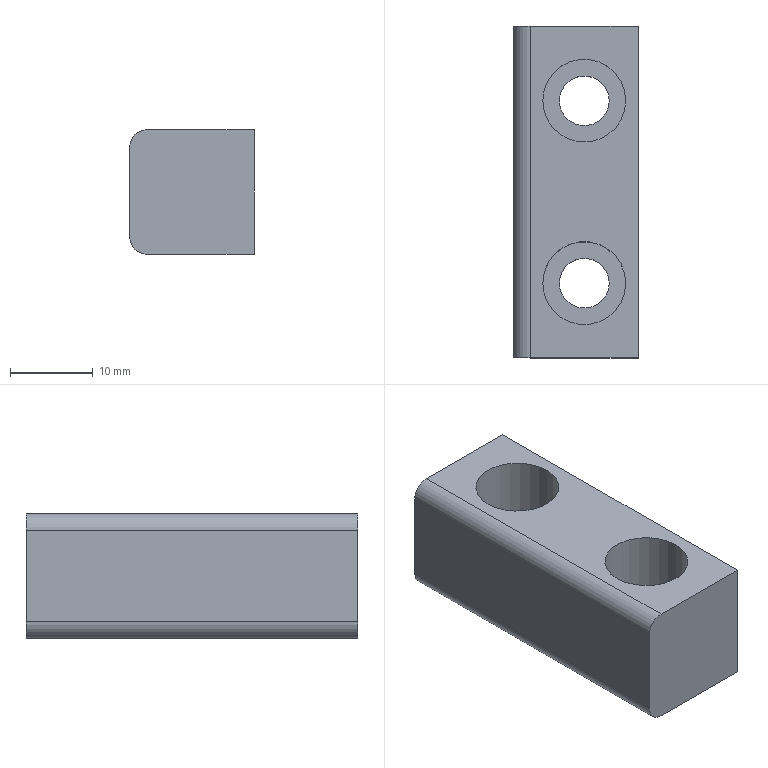Part | NX | features solid 2 | 1 solid | 14 faces | box 15 x 40 x 15 mm | volume 7279 mm3 | plane 8 | cylinder 6 | commonest cylinder face diameters 4 x2 6 x2 10 x2
STEP:
#1=CARTESIAN_POINT('',(496.902,-51.816,-17.));
#2=VERTEX_POINT('',#1);
#3=CARTESIAN_POINT('',(493.902,-51.816,-17.));
#4=DIRECTION('',(0.,0.,-1.));
#5=DIRECTION('',(1.,0.,0.));
#6=AXIS2_PLACEMENT_3D('',#3,#4,#5);
#7=CIRCLE('',#6,3.);
#8=EDGE_CURVE('',#2,#2,#7,.T.);
#9=ORIENTED_EDGE('',*,*,#8,.F.);
#10=EDGE_LOOP('',(#9));
#11=FACE_BOUND('',#10,.T.);
#12=CARTESIAN_POINT('',(487.402,-82.816,-17.));
#13=VERTEX_POINT('',#12);
#14=CARTESIAN_POINT('',(500.402,-82.816,-17.));
#15=VERTEX_POINT('',#14);
#16=CARTESIAN_POINT('',(490.402,-82.816,-17.));
#17=DIRECTION('',(1.,0.,0.));
#18=VECTOR('',#17,1000.);
#19=LINE('',#16,#18);
#20=EDGE_CURVE('',#13,#15,#19,.T.);
#21=ORIENTED_EDGE('',*,*,#20,.F.);
#22=CARTESIAN_POINT('',(487.402,-42.816,-17.));
#23=VERTEX_POINT('',#22);
#24=CARTESIAN_POINT('',(487.402,-62.816,-17.));
#25=DIRECTION('',(0.,-1.,0.));
#26=VECTOR('',#25,1000.);
#27=LINE('',#24,#26);
#28=EDGE_CURVE('',#13,#23,#27,.F.);
#29=ORIENTED_EDGE('',*,*,#28,.T.);
#30=CARTESIAN_POINT('',(500.402,-42.816,-17.));
#31=VERTEX_POINT('',#30);
#32=CARTESIAN_POINT('',(490.402,-42.816,-17.));
#33=DIRECTION('',(-1.,0.,0.));
#34=VECTOR('',#33,1000.);
#35=LINE('',#32,#34);
#36=EDGE_CURVE('',#31,#23,#35,.T.);
#37=ORIENTED_EDGE('',*,*,#36,.F.);
#38=CARTESIAN_POINT('',(500.402,-62.816,-17.));
#39=DIRECTION('',(0.,1.,0.));
#40=VECTOR('',#39,1000.);
#41=LINE('',#38,#40);
#42=EDGE_CURVE('',#15,#31,#41,.T.);
#43=ORIENTED_EDGE('',*,*,#42,.F.);
#44=EDGE_LOOP('',(#21,#29,#37,#43));
#45=FACE_BOUND('',#44,.T.);
#46=CARTESIAN_POINT('',(496.902,-73.816,-17.));
#47=VERTEX_POINT('',#46);
#48=CARTESIAN_POINT('',(493.902,-73.816,-17.));
#49=DIRECTION('',(0.,0.,1.));
#50=DIRECTION('',(1.,0.,0.));
#51=AXIS2_PLACEMENT_3D('',#48,#49,#50);
#52=CIRCLE('',#51,3.);
#53=EDGE_CURVE('',#47,#47,#52,.T.);
#54=ORIENTED_EDGE('',*,*,#53,.T.);
#55=EDGE_LOOP('',(#54));
#56=FACE_BOUND('',#55,.T.);
#57=CARTESIAN_POINT('',(490.402,-62.816,-17.));
#58=DIRECTION('',(0.,0.,-1.));
#59=DIRECTION('',(-1.,0.,0.));
#60=AXIS2_PLACEMENT_3D('',#57,#58,#59);
#61=PLANE('',#60);
#62=ADVANCED_FACE('',(#11,#45,#56),#61,.T.);
#63=CARTESIAN_POINT('',(498.902,-51.816,-2.));
#64=VERTEX_POINT('',#63);
#65=CARTESIAN_POINT('',(493.902,-51.816,-2.));
#66=DIRECTION('',(0.,0.,1.));
#67=DIRECTION('',(1.,0.,0.));
#68=AXIS2_PLACEMENT_3D('',#65,#66,#67);
#69=CIRCLE('',#68,5.);
#70=EDGE_CURVE('',#64,#64,#69,.T.);
#71=ORIENTED_EDGE('',*,*,#70,.F.);
#72=EDGE_LOOP('',(#71));
#73=FACE_BOUND('',#72,.T.);
#74=CARTESIAN_POINT('',(487.402,-42.816,-2.));
#75=VERTEX_POINT('',#74);
#76=CARTESIAN_POINT('',(500.402,-42.816,-2.));
#77=VERTEX_POINT('',#76);
#78=CARTESIAN_POINT('',(490.402,-42.816,-2.));
#79=DIRECTION('',(1.,0.,0.));
#80=VECTOR('',#79,1000.);
#81=LINE('',#78,#80);
#82=EDGE_CURVE('',#75,#77,#81,.T.);
#83=ORIENTED_EDGE('',*,*,#82,.F.);
#84=CARTESIAN_POINT('',(487.402,-82.816,-2.));
#85=VERTEX_POINT('',#84);
#86=CARTESIAN_POINT('',(487.402,-62.816,-2.));
#87=DIRECTION('',(0.,1.,0.));
#88=VECTOR('',#87,1000.);
#89=LINE('',#86,#88);
#90=EDGE_CURVE('',#75,#85,#89,.F.);
#91=ORIENTED_EDGE('',*,*,#90,.T.);
#92=CARTESIAN_POINT('',(500.402,-82.816,-2.));
#93=VERTEX_POINT('',#92);
#94=CARTESIAN_POINT('',(490.402,-82.816,-2.));
#95=DIRECTION('',(-1.,0.,0.));
#96=VECTOR('',#95,1000.);
#97=LINE('',#94,#96);
#98=EDGE_CURVE('',#93,#85,#97,.T.);
#99=ORIENTED_EDGE('',*,*,#98,.F.);
#100=CARTESIAN_POINT('',(500.402,-62.816,-2.));
#101=DIRECTION('',(0.,-1.,0.));
#102=VECTOR('',#101,1000.);
#103=LINE('',#100,#102);
#104=EDGE_CURVE('',#77,#93,#103,.T.);
#105=ORIENTED_EDGE('',*,*,#104,.F.);
#106=EDGE_LOOP('',(#83,#91,#99,#105));
#107=FACE_BOUND('',#106,.T.);
#108=CARTESIAN_POINT('',(498.902,-73.816,-2.));
#109=VERTEX_POINT('',#108);
#110=CARTESIAN_POINT('',(493.902,-73.816,-2.));
#111=DIRECTION('',(0.,0.,-1.));
#112=DIRECTION('',(1.,0.,0.));
#113=AXIS2_PLACEMENT_3D('',#110,#111,#112);
#114=CIRCLE('',#113,5.);
#115=EDGE_CURVE('',#109,#109,#114,.T.);
#116=ORIENTED_EDGE('',*,*,#115,.T.);
#117=EDGE_LOOP('',(#116));
#118=FACE_BOUND('',#117,.T.);
#119=CARTESIAN_POINT('',(490.402,-62.816,-2.));
#120=DIRECTION('',(0.,0.,1.));
#121=DIRECTION('',(1.,0.,0.));
#122=AXIS2_PLACEMENT_3D('',#119,#120,#121);
#123=PLANE('',#122);
#124=ADVANCED_FACE('',(#73,#107,#118),#123,.T.);
#125=CARTESIAN_POINT('',(485.402,-82.816,-15.));
#126=VERTEX_POINT('',#125);
#127=CARTESIAN_POINT('',(485.402,-82.816,-4.));
#128=VERTEX_POINT('',#127);
#129=CARTESIAN_POINT('',(485.402,-82.816,-12.));
#130=DIRECTION('',(0.,0.,1.));
#131=VECTOR('',#130,1000.);
#132=LINE('',#129,#131);
#133=EDGE_CURVE('',#126,#128,#132,.T.);
#134=ORIENTED_EDGE('',*,*,#133,.F.);
#135=CARTESIAN_POINT('',(487.402,-82.816,-15.));
#136=DIRECTION('',(0.,-1.,0.));
#137=DIRECTION('',(0.,0.,-1.));
#138=AXIS2_PLACEMENT_3D('',#135,#136,#137);
#139=CIRCLE('',#138,2.);
#140=EDGE_CURVE('',#126,#13,#139,.T.);
#141=ORIENTED_EDGE('',*,*,#140,.T.);
#142=ORIENTED_EDGE('',*,*,#20,.T.);
#143=CARTESIAN_POINT('',(500.402,-82.816,-12.));
#144=DIRECTION('',(0.,0.,1.));
#145=VECTOR('',#144,1000.);
#146=LINE('',#143,#145);
#147=EDGE_CURVE('',#15,#93,#146,.T.);
#148=ORIENTED_EDGE('',*,*,#147,.T.);
#149=ORIENTED_EDGE('',*,*,#98,.T.);
#150=CARTESIAN_POINT('',(487.402,-82.816,-4.));
#151=DIRECTION('',(0.,-1.,0.));
#152=DIRECTION('',(0.,0.,-1.));
#153=AXIS2_PLACEMENT_3D('',#150,#151,#152);
#154=CIRCLE('',#153,2.);
#155=EDGE_CURVE('',#85,#128,#154,.T.);
#156=ORIENTED_EDGE('',*,*,#155,.T.);
#157=EDGE_LOOP('',(#134,#141,#142,#148,#149,#156));
#158=FACE_BOUND('',#157,.T.);
#159=CARTESIAN_POINT('',(490.402,-82.816,-12.));
#160=DIRECTION('',(0.,-1.,0.));
#161=DIRECTION('',(0.,0.,-1.));
#162=AXIS2_PLACEMENT_3D('',#159,#160,#161);
#163=PLANE('',#162);
#164=ADVANCED_FACE('',(#158),#163,.T.);
#165=CARTESIAN_POINT('',(485.402,-42.816,-15.));
#166=VERTEX_POINT('',#165);
#167=CARTESIAN_POINT('',(485.402,-42.816,-4.));
#168=VERTEX_POINT('',#167);
#169=CARTESIAN_POINT('',(485.402,-42.816,-12.));
#170=DIRECTION('',(0.,0.,1.));
#171=VECTOR('',#170,1000.);
#172=LINE('',#169,#171);
#173=EDGE_CURVE('',#166,#168,#172,.T.);
#174=ORIENTED_EDGE('',*,*,#173,.F.);
#175=CARTESIAN_POINT('',(485.402,-62.816,-15.));
#176=DIRECTION('',(0.,-1.,0.));
#177=VECTOR('',#176,1000.);
#178=LINE('',#175,#177);
#179=EDGE_CURVE('',#166,#126,#178,.T.);
#180=ORIENTED_EDGE('',*,*,#179,.T.);
#181=ORIENTED_EDGE('',*,*,#133,.T.);
#182=CARTESIAN_POINT('',(485.402,-62.816,-4.));
#183=DIRECTION('',(0.,1.,0.));
#184=VECTOR('',#183,1000.);
#185=LINE('',#182,#184);
#186=EDGE_CURVE('',#128,#168,#185,.T.);
#187=ORIENTED_EDGE('',*,*,#186,.T.);
#188=EDGE_LOOP('',(#174,#180,#181,#187));
#189=FACE_BOUND('',#188,.T.);
#190=CARTESIAN_POINT('',(485.402,-62.816,-12.));
#191=DIRECTION('',(-1.,0.,0.));
#192=DIRECTION('',(0.,0.,1.));
#193=AXIS2_PLACEMENT_3D('',#190,#191,#192);
#194=PLANE('',#193);
#195=ADVANCED_FACE('',(#189),#194,.T.);
#196=ORIENTED_EDGE('',*,*,#36,.T.);
#197=CARTESIAN_POINT('',(487.402,-42.816,-15.));
#198=DIRECTION('',(0.,1.,0.));
#199=DIRECTION('',(0.,0.,1.));
#200=AXIS2_PLACEMENT_3D('',#197,#198,#199);
#201=CIRCLE('',#200,2.);
#202=EDGE_CURVE('',#23,#166,#201,.T.);
#203=ORIENTED_EDGE('',*,*,#202,.T.);
#204=ORIENTED_EDGE('',*,*,#173,.T.);
#205=CARTESIAN_POINT('',(487.402,-42.816,-4.));
#206=DIRECTION('',(0.,1.,0.));
#207=DIRECTION('',(0.,0.,1.));
#208=AXIS2_PLACEMENT_3D('',#205,#206,#207);
#209=CIRCLE('',#208,2.);
#210=EDGE_CURVE('',#168,#75,#209,.T.);
#211=ORIENTED_EDGE('',*,*,#210,.T.);
#212=ORIENTED_EDGE('',*,*,#82,.T.);
#213=CARTESIAN_POINT('',(500.402,-42.816,-12.));
#214=DIRECTION('',(0.,0.,1.));
#215=VECTOR('',#214,1000.);
#216=LINE('',#213,#215);
#217=EDGE_CURVE('',#31,#77,#216,.T.);
#218=ORIENTED_EDGE('',*,*,#217,.F.);
#219=EDGE_LOOP('',(#196,#203,#204,#211,#212,#218));
#220=FACE_BOUND('',#219,.T.);
#221=CARTESIAN_POINT('',(490.402,-42.816,-12.));
#222=DIRECTION('',(0.,1.,0.));
#223=DIRECTION('',(0.,0.,1.));
#224=AXIS2_PLACEMENT_3D('',#221,#222,#223);
#225=PLANE('',#224);
#226=ADVANCED_FACE('',(#220),#225,.T.);
#227=ORIENTED_EDGE('',*,*,#42,.T.);
#228=ORIENTED_EDGE('',*,*,#217,.T.);
#229=ORIENTED_EDGE('',*,*,#104,.T.);
#230=ORIENTED_EDGE('',*,*,#147,.F.);
#231=EDGE_LOOP('',(#227,#228,#229,#230));
#232=FACE_BOUND('',#231,.T.);
#233=CARTESIAN_POINT('',(500.402,-62.816,-12.));
#234=DIRECTION('',(1.,0.,0.));
#235=DIRECTION('',(0.,0.,-1.));
#236=AXIS2_PLACEMENT_3D('',#233,#234,#235);
#237=PLANE('',#236);
#238=ADVANCED_FACE('',(#232),#237,.T.);
#239=ORIENTED_EDGE('',*,*,#202,.F.);
#240=ORIENTED_EDGE('',*,*,#28,.F.);
#241=ORIENTED_EDGE('',*,*,#140,.F.);
#242=ORIENTED_EDGE('',*,*,#179,.F.);
#243=EDGE_LOOP('',(#239,#240,#241,#242));
#244=FACE_BOUND('',#243,.T.);
#245=CARTESIAN_POINT('',(487.402,-62.816,-15.));
#246=DIRECTION('',(0.,-1.,0.));
#247=DIRECTION('',(0.,0.,-1.));
#248=AXIS2_PLACEMENT_3D('',#245,#246,#247);
#249=CYLINDRICAL_SURFACE('',#248,2.);
#250=ADVANCED_FACE('',(#244),#249,.T.);
#251=ORIENTED_EDGE('',*,*,#155,.F.);
#252=ORIENTED_EDGE('',*,*,#90,.F.);
#253=ORIENTED_EDGE('',*,*,#210,.F.);
#254=ORIENTED_EDGE('',*,*,#186,.F.);
#255=EDGE_LOOP('',(#251,#252,#253,#254));
#256=FACE_BOUND('',#255,.T.);
#257=CARTESIAN_POINT('',(487.402,-62.816,-4.));
#258=DIRECTION('',(0.,1.,0.));
#259=DIRECTION('',(0.,0.,1.));
#260=AXIS2_PLACEMENT_3D('',#257,#258,#259);
#261=CYLINDRICAL_SURFACE('',#260,2.);
#262=ADVANCED_FACE('',(#256),#261,.T.);
#263=CARTESIAN_POINT('',(490.902,-73.816,-10.));
#264=VERTEX_POINT('',#263);
#265=CARTESIAN_POINT('',(493.902,-73.816,-10.));
#266=DIRECTION('',(0.,0.,-1.));
#267=DIRECTION('',(-1.,0.,0.));
#268=AXIS2_PLACEMENT_3D('',#265,#266,#267);
#269=CIRCLE('',#268,3.);
#270=EDGE_CURVE('',#264,#264,#269,.T.);
#271=ORIENTED_EDGE('',*,*,#270,.F.);
#272=EDGE_LOOP('',(#271));
#273=FACE_BOUND('',#272,.T.);
#274=ORIENTED_EDGE('',*,*,#53,.F.);
#275=EDGE_LOOP('',(#274));
#276=FACE_BOUND('',#275,.T.);
#277=CARTESIAN_POINT('',(493.902,-73.816,-2.));
#278=DIRECTION('',(0.,0.,-1.));
#279=DIRECTION('',(1.,0.,0.));
#280=AXIS2_PLACEMENT_3D('',#277,#278,#279);
#281=CYLINDRICAL_SURFACE('',#280,3.);
#282=ADVANCED_FACE('',(#273,#276),#281,.F.);
#283=ORIENTED_EDGE('',*,*,#270,.T.);
#284=EDGE_LOOP('',(#283));
#285=FACE_BOUND('',#284,.T.);
#286=CARTESIAN_POINT('',(498.902,-73.816,-10.));
#287=VERTEX_POINT('',#286);
#288=CARTESIAN_POINT('',(493.902,-73.816,-10.));
#289=DIRECTION('',(0.,0.,1.));
#290=DIRECTION('',(1.,0.,0.));
#291=AXIS2_PLACEMENT_3D('',#288,#289,#290);
#292=CIRCLE('',#291,5.);
#293=EDGE_CURVE('',#287,#287,#292,.F.);
#294=ORIENTED_EDGE('',*,*,#293,.F.);
#295=EDGE_LOOP('',(#294));
#296=FACE_BOUND('',#295,.T.);
#297=CARTESIAN_POINT('',(493.902,-73.816,-10.));
#298=DIRECTION('',(0.,0.,-1.));
#299=DIRECTION('',(-1.,0.,0.));
#300=AXIS2_PLACEMENT_3D('',#297,#298,#299);
#301=PLANE('',#300);
#302=ADVANCED_FACE('',(#285,#296),#301,.F.);
#303=ORIENTED_EDGE('',*,*,#293,.T.);
#304=EDGE_LOOP('',(#303));
#305=FACE_BOUND('',#304,.T.);
#306=ORIENTED_EDGE('',*,*,#115,.F.);
#307=EDGE_LOOP('',(#306));
#308=FACE_BOUND('',#307,.T.);
#309=CARTESIAN_POINT('',(493.902,-73.816,-2.));
#310=DIRECTION('',(0.,0.,-1.));
#311=DIRECTION('',(1.,0.,0.));
#312=AXIS2_PLACEMENT_3D('',#309,#310,#311);
#313=CYLINDRICAL_SURFACE('',#312,5.);
#314=ADVANCED_FACE('',(#305,#308),#313,.F.);
#315=CARTESIAN_POINT('',(490.902,-51.816,-10.));
#316=VERTEX_POINT('',#315);
#317=CARTESIAN_POINT('',(493.902,-51.816,-10.));
#318=DIRECTION('',(0.,0.,1.));
#319=DIRECTION('',(-1.,0.,0.));
#320=AXIS2_PLACEMENT_3D('',#317,#318,#319);
#321=CIRCLE('',#320,3.);
#322=EDGE_CURVE('',#316,#316,#321,.T.);
#323=ORIENTED_EDGE('',*,*,#322,.T.);
#324=EDGE_LOOP('',(#323));
#325=FACE_BOUND('',#324,.T.);
#326=ORIENTED_EDGE('',*,*,#8,.T.);
#327=EDGE_LOOP('',(#326));
#328=FACE_BOUND('',#327,.T.);
#329=CARTESIAN_POINT('',(493.902,-51.816,-2.));
#330=DIRECTION('',(0.,0.,-1.));
#331=DIRECTION('',(1.,0.,0.));
#332=AXIS2_PLACEMENT_3D('',#329,#330,#331);
#333=CYLINDRICAL_SURFACE('',#332,3.);
#334=ADVANCED_FACE('',(#325,#328),#333,.F.);
#335=ORIENTED_EDGE('',*,*,#322,.F.);
#336=EDGE_LOOP('',(#335));
#337=FACE_BOUND('',#336,.T.);
#338=CARTESIAN_POINT('',(498.902,-51.816,-10.));
#339=VERTEX_POINT('',#338);
#340=CARTESIAN_POINT('',(493.902,-51.816,-10.));
#341=DIRECTION('',(0.,0.,-1.));
#342=DIRECTION('',(1.,0.,0.));
#343=AXIS2_PLACEMENT_3D('',#340,#341,#342);
#344=CIRCLE('',#343,5.);
#345=EDGE_CURVE('',#339,#339,#344,.F.);
#346=ORIENTED_EDGE('',*,*,#345,.T.);
#347=EDGE_LOOP('',(#346));
#348=FACE_BOUND('',#347,.T.);
#349=CARTESIAN_POINT('',(493.902,-51.816,-10.));
#350=DIRECTION('',(0.,0.,-1.));
#351=DIRECTION('',(-1.,0.,0.));
#352=AXIS2_PLACEMENT_3D('',#349,#350,#351);
#353=PLANE('',#352);
#354=ADVANCED_FACE('',(#337,#348),#353,.F.);
#355=ORIENTED_EDGE('',*,*,#345,.F.);
#356=EDGE_LOOP('',(#355));
#357=FACE_BOUND('',#356,.T.);
#358=ORIENTED_EDGE('',*,*,#70,.T.);
#359=EDGE_LOOP('',(#358));
#360=FACE_BOUND('',#359,.T.);
#361=CARTESIAN_POINT('',(493.902,-51.816,-2.));
#362=DIRECTION('',(0.,0.,-1.));
#363=DIRECTION('',(1.,0.,0.));
#364=AXIS2_PLACEMENT_3D('',#361,#362,#363);
#365=CYLINDRICAL_SURFACE('',#364,5.);
#366=ADVANCED_FACE('',(#357,#360),#365,.F.);
#367=CLOSED_SHELL('',(#62,#124,#164,#195,#226,#238,#250,#262,#282,#302,#314,#334,#354,#366));
#368=MANIFOLD_SOLID_BREP('',#367);
#369=(LENGTH_UNIT()NAMED_UNIT(*)SI_UNIT(.MILLI.,.METRE.));
#370=UNCERTAINTY_MEASURE_WITH_UNIT(LENGTH_MEASURE(0.00001),#369,'','');
#371=(NAMED_UNIT(*)PLANE_ANGLE_UNIT()SI_UNIT($,.RADIAN.));
#372=(NAMED_UNIT(*)SI_UNIT($,.STERADIAN.)SOLID_ANGLE_UNIT());
#373=(GEOMETRIC_REPRESENTATION_CONTEXT(3)GLOBAL_UNCERTAINTY_ASSIGNED_CONTEXT((#370))GLOBAL_UNIT_ASSIGNED_CONTEXT((#369,#371,#372))REPRESENTATION_CONTEXT('',''));
#374=ADVANCED_BREP_SHAPE_REPRESENTATION('',(#368),#373);